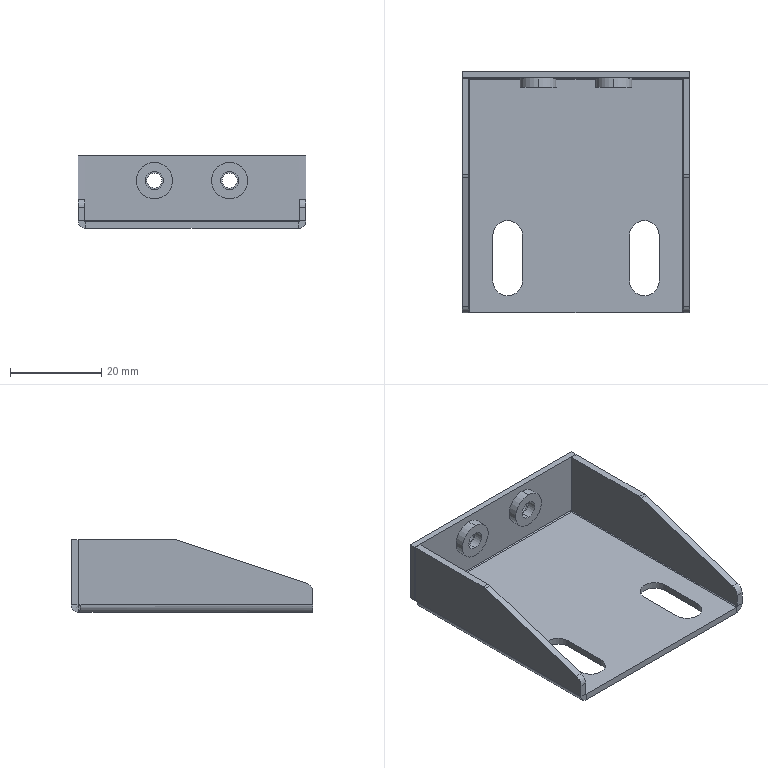Part | STEP file | Door hinge mounting plate | 1 solid | 64 faces | box 50 x 53 x 16 mm | volume 6575 mm3 | plane 34 | cylinder 26 | spline 4 | commonest cylinder face diameters 4 x8 3.3 x4 6.5 x4 8 x4 0.4 x3 3.4 x3